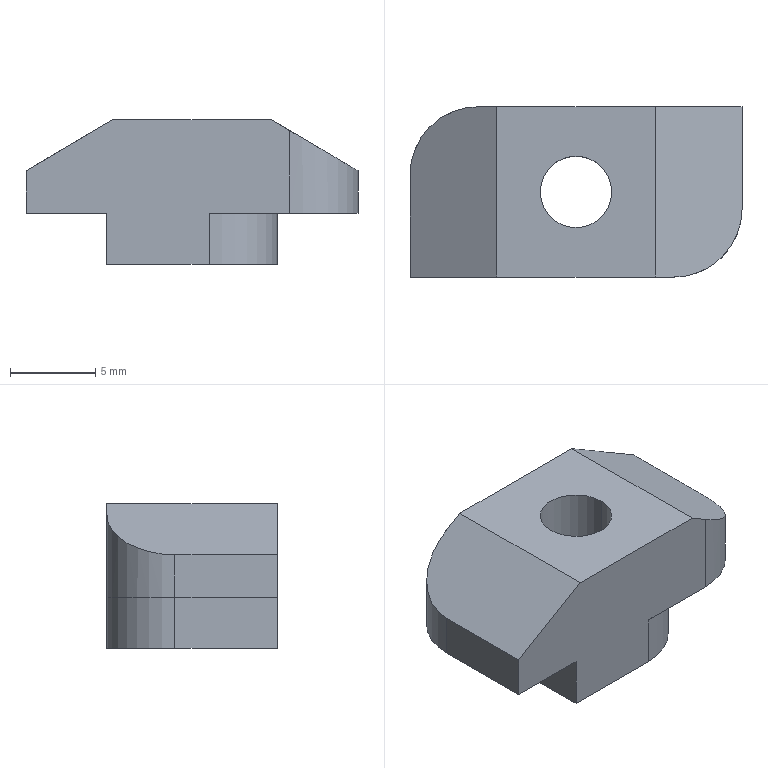Part | NX | features BREP 1 | 1 solid | 18 faces | box 19.5 x 10 x 8.5 mm | volume 1060 mm3 | plane 12 | cylinder 6 | commonest cylinder face diameters 8 x4 4.2 x2
STEP:
#1=CARTESIAN_POINT('',(-2.1,0.,-8.5));
#2=VERTEX_POINT('',#1);
#3=CARTESIAN_POINT('',(2.1,0.,-8.5));
#4=VERTEX_POINT('',#3);
#5=CARTESIAN_POINT('',(0.,0.,-8.5));
#6=DIRECTION('',(0.,0.,-1.));
#7=DIRECTION('',(-1.,0.,0.));
#8=AXIS2_PLACEMENT_3D('',#5,#6,#7);
#9=CIRCLE('',#8,2.1);
#10=EDGE_CURVE('',#2,#4,#9,.T.);
#11=ORIENTED_EDGE('',*,*,#10,.T.);
#12=CARTESIAN_POINT('',(2.1,0.,0.));
#13=VERTEX_POINT('',#12);
#14=CARTESIAN_POINT('',(2.1,0.,0.));
#15=DIRECTION('',(0.,0.,1.));
#16=VECTOR('',#15,1000.);
#17=LINE('',#14,#16);
#18=EDGE_CURVE('',#4,#13,#17,.T.);
#19=ORIENTED_EDGE('',*,*,#18,.T.);
#20=CARTESIAN_POINT('',(-2.1,0.,0.));
#21=VERTEX_POINT('',#20);
#22=CARTESIAN_POINT('',(0.,0.,0.));
#23=DIRECTION('',(0.,0.,-1.));
#24=DIRECTION('',(-1.,0.,0.));
#25=AXIS2_PLACEMENT_3D('',#22,#23,#24);
#26=CIRCLE('',#25,2.1);
#27=EDGE_CURVE('',#21,#13,#26,.T.);
#28=ORIENTED_EDGE('',*,*,#27,.F.);
#29=CARTESIAN_POINT('',(-2.1,0.,0.));
#30=DIRECTION('',(0.,0.,1.));
#31=VECTOR('',#30,1000.);
#32=LINE('',#29,#31);
#33=EDGE_CURVE('',#2,#21,#32,.T.);
#34=ORIENTED_EDGE('',*,*,#33,.F.);
#35=EDGE_LOOP('',(#11,#19,#28,#34));
#36=FACE_BOUND('',#35,.T.);
#37=CARTESIAN_POINT('',(0.,0.,0.));
#38=DIRECTION('',(0.,0.,1.));
#39=DIRECTION('',(-1.,0.,0.));
#40=AXIS2_PLACEMENT_3D('',#37,#38,#39);
#41=CYLINDRICAL_SURFACE('',#40,2.1);
#42=ADVANCED_FACE('',(#36),#41,.F.);
#43=CARTESIAN_POINT('',(1.,-5.,-5.5));
#44=VERTEX_POINT('',#43);
#45=CARTESIAN_POINT('',(5.75,-5.,-5.5));
#46=VERTEX_POINT('',#45);
#47=CARTESIAN_POINT('',(-9.75,-5.,-5.5));
#48=DIRECTION('',(1.,0.,0.));
#49=VECTOR('',#48,1000.);
#50=LINE('',#47,#49);
#51=EDGE_CURVE('',#44,#46,#50,.T.);
#52=ORIENTED_EDGE('',*,*,#51,.F.);
#53=CARTESIAN_POINT('',(5.,-1.,-5.5));
#54=VERTEX_POINT('',#53);
#55=CARTESIAN_POINT('',(1.,-1.,-5.5));
#56=DIRECTION('',(0.,0.,-1.));
#57=DIRECTION('',(1.,0.,0.));
#58=AXIS2_PLACEMENT_3D('',#55,#56,#57);
#59=CIRCLE('',#58,4.);
#60=EDGE_CURVE('',#54,#44,#59,.T.);
#61=ORIENTED_EDGE('',*,*,#60,.F.);
#62=CARTESIAN_POINT('',(5.,5.,-5.5));
#63=VERTEX_POINT('',#62);
#64=CARTESIAN_POINT('',(5.,-5.,-5.5));
#65=DIRECTION('',(0.,1.,0.));
#66=VECTOR('',#65,1000.);
#67=LINE('',#64,#66);
#68=EDGE_CURVE('',#54,#63,#67,.T.);
#69=ORIENTED_EDGE('',*,*,#68,.T.);
#70=CARTESIAN_POINT('',(9.75,5.,-5.5));
#71=VERTEX_POINT('',#70);
#72=CARTESIAN_POINT('',(-9.75,5.,-5.5));
#73=DIRECTION('',(-1.,0.,0.));
#74=VECTOR('',#73,1000.);
#75=LINE('',#72,#74);
#76=EDGE_CURVE('',#71,#63,#75,.T.);
#77=ORIENTED_EDGE('',*,*,#76,.F.);
#78=CARTESIAN_POINT('',(9.75,-1.,-5.5));
#79=VERTEX_POINT('',#78);
#80=CARTESIAN_POINT('',(9.75,5.,-5.5));
#81=DIRECTION('',(0.,1.,0.));
#82=VECTOR('',#81,1000.);
#83=LINE('',#80,#82);
#84=EDGE_CURVE('',#79,#71,#83,.T.);
#85=ORIENTED_EDGE('',*,*,#84,.F.);
#86=CARTESIAN_POINT('',(5.75,-1.,-5.5));
#87=DIRECTION('',(0.,0.,1.));
#88=DIRECTION('',(1.,0.,0.));
#89=AXIS2_PLACEMENT_3D('',#86,#87,#88);
#90=CIRCLE('',#89,4.);
#91=EDGE_CURVE('',#46,#79,#90,.T.);
#92=ORIENTED_EDGE('',*,*,#91,.F.);
#93=EDGE_LOOP('',(#52,#61,#69,#77,#85,#92));
#94=FACE_BOUND('',#93,.T.);
#95=CARTESIAN_POINT('',(0.,0.,-5.5));
#96=DIRECTION('',(0.,0.,-1.));
#97=DIRECTION('',(0.,-1.,0.));
#98=AXIS2_PLACEMENT_3D('',#95,#96,#97);
#99=PLANE('',#98);
#100=ADVANCED_FACE('',(#94),#99,.T.);
#101=ORIENTED_EDGE('',*,*,#84,.T.);
#102=CARTESIAN_POINT('',(9.75,5.,-3.));
#103=VERTEX_POINT('',#102);
#104=CARTESIAN_POINT('',(9.75,5.,-5.5));
#105=DIRECTION('',(0.,0.,1.));
#106=VECTOR('',#105,1000.);
#107=LINE('',#104,#106);
#108=EDGE_CURVE('',#71,#103,#107,.T.);
#109=ORIENTED_EDGE('',*,*,#108,.T.);
#110=CARTESIAN_POINT('',(9.75,-1.,-3.));
#111=VERTEX_POINT('',#110);
#112=CARTESIAN_POINT('',(9.75,5.,-3.));
#113=DIRECTION('',(0.,1.,0.));
#114=VECTOR('',#113,1000.);
#115=LINE('',#112,#114);
#116=EDGE_CURVE('',#111,#103,#115,.T.);
#117=ORIENTED_EDGE('',*,*,#116,.F.);
#118=CARTESIAN_POINT('',(9.75,-1.,-5.5));
#119=DIRECTION('',(0.,0.,1.));
#120=VECTOR('',#119,1000.);
#121=LINE('',#118,#120);
#122=EDGE_CURVE('',#79,#111,#121,.T.);
#123=ORIENTED_EDGE('',*,*,#122,.F.);
#124=EDGE_LOOP('',(#101,#109,#117,#123));
#125=FACE_BOUND('',#124,.T.);
#126=CARTESIAN_POINT('',(9.75,5.,-5.5));
#127=DIRECTION('',(-1.,0.,0.));
#128=DIRECTION('',(0.,1.,0.));
#129=AXIS2_PLACEMENT_3D('',#126,#127,#128);
#130=PLANE('',#129);
#131=ADVANCED_FACE('',(#125),#130,.F.);
#132=CARTESIAN_POINT('',(-4.65,5.,0.));
#133=VERTEX_POINT('',#132);
#134=CARTESIAN_POINT('',(-5.75,5.,-0.6471));
#135=VERTEX_POINT('',#134);
#136=CARTESIAN_POINT('',(-9.75,5.,-3.));
#137=DIRECTION('',(-0.8619,0.,-0.507));
#138=VECTOR('',#137,1000.);
#139=LINE('',#136,#138);
#140=EDGE_CURVE('',#133,#135,#139,.T.);
#141=ORIENTED_EDGE('',*,*,#140,.F.);
#142=CARTESIAN_POINT('',(4.65,5.,0.));
#143=VERTEX_POINT('',#142);
#144=CARTESIAN_POINT('',(-9.75,5.,0.));
#145=DIRECTION('',(-1.,0.,0.));
#146=VECTOR('',#145,1000.);
#147=LINE('',#144,#146);
#148=EDGE_CURVE('',#143,#133,#147,.T.);
#149=ORIENTED_EDGE('',*,*,#148,.F.);
#150=CARTESIAN_POINT('',(9.75,5.,-3.));
#151=DIRECTION('',(-0.8619,0.,0.507));
#152=VECTOR('',#151,1000.);
#153=LINE('',#150,#152);
#154=EDGE_CURVE('',#103,#143,#153,.T.);
#155=ORIENTED_EDGE('',*,*,#154,.F.);
#156=ORIENTED_EDGE('',*,*,#108,.F.);
#157=ORIENTED_EDGE('',*,*,#76,.T.);
#158=CARTESIAN_POINT('',(5.,5.,-8.5));
#159=VERTEX_POINT('',#158);
#160=CARTESIAN_POINT('',(5.,5.,-8.5));
#161=DIRECTION('',(0.,0.,1.));
#162=VECTOR('',#161,1000.);
#163=LINE('',#160,#162);
#164=EDGE_CURVE('',#159,#63,#163,.T.);
#165=ORIENTED_EDGE('',*,*,#164,.F.);
#166=CARTESIAN_POINT('',(-1.,5.,-8.5));
#167=VERTEX_POINT('',#166);
#168=CARTESIAN_POINT('',(-5.,5.,-8.5));
#169=DIRECTION('',(-1.,0.,0.));
#170=VECTOR('',#169,1000.);
#171=LINE('',#168,#170);
#172=EDGE_CURVE('',#159,#167,#171,.T.);
#173=ORIENTED_EDGE('',*,*,#172,.T.);
#174=CARTESIAN_POINT('',(-1.,5.,-5.5));
#175=VERTEX_POINT('',#174);
#176=CARTESIAN_POINT('',(-1.,5.,-5.5));
#177=DIRECTION('',(0.,0.,-1.));
#178=VECTOR('',#177,1000.);
#179=LINE('',#176,#178);
#180=EDGE_CURVE('',#175,#167,#179,.T.);
#181=ORIENTED_EDGE('',*,*,#180,.F.);
#182=CARTESIAN_POINT('',(-5.75,5.,-5.5));
#183=VERTEX_POINT('',#182);
#184=CARTESIAN_POINT('',(-9.75,5.,-5.5));
#185=DIRECTION('',(-1.,0.,0.));
#186=VECTOR('',#185,1000.);
#187=LINE('',#184,#186);
#188=EDGE_CURVE('',#175,#183,#187,.T.);
#189=ORIENTED_EDGE('',*,*,#188,.T.);
#190=CARTESIAN_POINT('',(-5.75,5.,-5.5));
#191=DIRECTION('',(0.,0.,-1.));
#192=VECTOR('',#191,1000.);
#193=LINE('',#190,#192);
#194=EDGE_CURVE('',#135,#183,#193,.T.);
#195=ORIENTED_EDGE('',*,*,#194,.F.);
#196=EDGE_LOOP('',(#141,#149,#155,#156,#157,#165,#173,#181,#189,#195));
#197=FACE_BOUND('',#196,.T.);
#198=CARTESIAN_POINT('',(-9.75,5.,-5.5));
#199=DIRECTION('',(0.,-1.,0.));
#200=DIRECTION('',(0.,0.,-1.));
#201=AXIS2_PLACEMENT_3D('',#198,#199,#200);
#202=PLANE('',#201);
#203=ADVANCED_FACE('',(#197),#202,.F.);
#204=CARTESIAN_POINT('',(-9.75,1.,-5.5));
#205=VERTEX_POINT('',#204);
#206=CARTESIAN_POINT('',(-9.75,-5.,-5.5));
#207=VERTEX_POINT('',#206);
#208=CARTESIAN_POINT('',(-9.75,5.,-5.5));
#209=DIRECTION('',(0.,-1.,0.));
#210=VECTOR('',#209,1000.);
#211=LINE('',#208,#210);
#212=EDGE_CURVE('',#205,#207,#211,.T.);
#213=ORIENTED_EDGE('',*,*,#212,.T.);
#214=CARTESIAN_POINT('',(-9.75,-5.,-3.));
#215=VERTEX_POINT('',#214);
#216=CARTESIAN_POINT('',(-9.75,-5.,-5.5));
#217=DIRECTION('',(0.,0.,1.));
#218=VECTOR('',#217,1000.);
#219=LINE('',#216,#218);
#220=EDGE_CURVE('',#207,#215,#219,.T.);
#221=ORIENTED_EDGE('',*,*,#220,.T.);
#222=CARTESIAN_POINT('',(-9.75,1.,-3.));
#223=VERTEX_POINT('',#222);
#224=CARTESIAN_POINT('',(-9.75,5.,-3.));
#225=DIRECTION('',(0.,-1.,0.));
#226=VECTOR('',#225,1000.);
#227=LINE('',#224,#226);
#228=EDGE_CURVE('',#223,#215,#227,.T.);
#229=ORIENTED_EDGE('',*,*,#228,.F.);
#230=CARTESIAN_POINT('',(-9.75,1.,-5.5));
#231=DIRECTION('',(0.,0.,1.));
#232=VECTOR('',#231,1000.);
#233=LINE('',#230,#232);
#234=EDGE_CURVE('',#205,#223,#233,.T.);
#235=ORIENTED_EDGE('',*,*,#234,.F.);
#236=EDGE_LOOP('',(#213,#221,#229,#235));
#237=FACE_BOUND('',#236,.T.);
#238=CARTESIAN_POINT('',(-9.75,5.,-5.5));
#239=DIRECTION('',(1.,0.,0.));
#240=DIRECTION('',(0.,1.,0.));
#241=AXIS2_PLACEMENT_3D('',#238,#239,#240);
#242=PLANE('',#241);
#243=ADVANCED_FACE('',(#237),#242,.F.);
#244=CARTESIAN_POINT('',(4.65,-5.,0.));
#245=VERTEX_POINT('',#244);
#246=CARTESIAN_POINT('',(5.75,-5.,-0.6471));
#247=VERTEX_POINT('',#246);
#248=CARTESIAN_POINT('',(9.75,-5.,-3.));
#249=DIRECTION('',(0.8619,0.,-0.507));
#250=VECTOR('',#249,1000.);
#251=LINE('',#248,#250);
#252=EDGE_CURVE('',#245,#247,#251,.T.);
#253=ORIENTED_EDGE('',*,*,#252,.F.);
#254=CARTESIAN_POINT('',(-4.65,-5.,0.));
#255=VERTEX_POINT('',#254);
#256=CARTESIAN_POINT('',(-9.75,-5.,0.));
#257=DIRECTION('',(1.,0.,0.));
#258=VECTOR('',#257,1000.);
#259=LINE('',#256,#258);
#260=EDGE_CURVE('',#255,#245,#259,.T.);
#261=ORIENTED_EDGE('',*,*,#260,.F.);
#262=CARTESIAN_POINT('',(-9.75,-5.,-3.));
#263=DIRECTION('',(0.8619,0.,0.507));
#264=VECTOR('',#263,1000.);
#265=LINE('',#262,#264);
#266=EDGE_CURVE('',#215,#255,#265,.T.);
#267=ORIENTED_EDGE('',*,*,#266,.F.);
#268=ORIENTED_EDGE('',*,*,#220,.F.);
#269=CARTESIAN_POINT('',(-5.,-5.,-5.5));
#270=VERTEX_POINT('',#269);
#271=CARTESIAN_POINT('',(-9.75,-5.,-5.5));
#272=DIRECTION('',(1.,0.,0.));
#273=VECTOR('',#272,1000.);
#274=LINE('',#271,#273);
#275=EDGE_CURVE('',#207,#270,#274,.T.);
#276=ORIENTED_EDGE('',*,*,#275,.T.);
#277=CARTESIAN_POINT('',(-5.,-5.,-8.5));
#278=VERTEX_POINT('',#277);
#279=CARTESIAN_POINT('',(-5.,-5.,-8.5));
#280=DIRECTION('',(0.,0.,1.));
#281=VECTOR('',#280,1000.);
#282=LINE('',#279,#281);
#283=EDGE_CURVE('',#278,#270,#282,.T.);
#284=ORIENTED_EDGE('',*,*,#283,.F.);
#285=CARTESIAN_POINT('',(1.,-5.,-8.5));
#286=VERTEX_POINT('',#285);
#287=CARTESIAN_POINT('',(-5.,-5.,-8.5));
#288=DIRECTION('',(1.,0.,0.));
#289=VECTOR('',#288,1000.);
#290=LINE('',#287,#289);
#291=EDGE_CURVE('',#278,#286,#290,.T.);
#292=ORIENTED_EDGE('',*,*,#291,.T.);
#293=CARTESIAN_POINT('',(1.,-5.,-5.5));
#294=DIRECTION('',(0.,0.,-1.));
#295=VECTOR('',#294,1000.);
#296=LINE('',#293,#295);
#297=EDGE_CURVE('',#44,#286,#296,.T.);
#298=ORIENTED_EDGE('',*,*,#297,.F.);
#299=ORIENTED_EDGE('',*,*,#51,.T.);
#300=CARTESIAN_POINT('',(5.75,-5.,-5.5));
#301=DIRECTION('',(0.,0.,-1.));
#302=VECTOR('',#301,1000.);
#303=LINE('',#300,#302);
#304=EDGE_CURVE('',#247,#46,#303,.T.);
#305=ORIENTED_EDGE('',*,*,#304,.F.);
#306=EDGE_LOOP('',(#253,#261,#267,#268,#276,#284,#292,#298,#299,#305));
#307=FACE_BOUND('',#306,.T.);
#308=CARTESIAN_POINT('',(-9.75,-5.,-5.5));
#309=DIRECTION('',(0.,1.,0.));
#310=DIRECTION('',(1.,0.,0.));
#311=AXIS2_PLACEMENT_3D('',#308,#309,#310);
#312=PLANE('',#311);
#313=ADVANCED_FACE('',(#307),#312,.F.);
#314=ORIENTED_EDGE('',*,*,#188,.F.);
#315=CARTESIAN_POINT('',(-5.,1.,-5.5));
#316=VERTEX_POINT('',#315);
#317=CARTESIAN_POINT('',(-1.,1.,-5.5));
#318=DIRECTION('',(0.,0.,-1.));
#319=DIRECTION('',(1.,0.,0.));
#320=AXIS2_PLACEMENT_3D('',#317,#318,#319);
#321=CIRCLE('',#320,4.);
#322=EDGE_CURVE('',#316,#175,#321,.T.);
#323=ORIENTED_EDGE('',*,*,#322,.F.);
#324=CARTESIAN_POINT('',(-5.,-5.,-5.5));
#325=DIRECTION('',(0.,-1.,0.));
#326=VECTOR('',#325,1000.);
#327=LINE('',#324,#326);
#328=EDGE_CURVE('',#316,#270,#327,.T.);
#329=ORIENTED_EDGE('',*,*,#328,.T.);
#330=ORIENTED_EDGE('',*,*,#275,.F.);
#331=ORIENTED_EDGE('',*,*,#212,.F.);
#332=CARTESIAN_POINT('',(-5.75,1.,-5.5));
#333=DIRECTION('',(0.,0.,1.));
#334=DIRECTION('',(1.,0.,0.));
#335=AXIS2_PLACEMENT_3D('',#332,#333,#334);
#336=CIRCLE('',#335,4.);
#337=EDGE_CURVE('',#183,#205,#336,.T.);
#338=ORIENTED_EDGE('',*,*,#337,.F.);
#339=EDGE_LOOP('',(#314,#323,#329,#330,#331,#338));
#340=FACE_BOUND('',#339,.T.);
#341=CARTESIAN_POINT('',(0.,0.,-5.5));
#342=DIRECTION('',(0.,0.,-1.));
#343=DIRECTION('',(0.,-1.,0.));
#344=AXIS2_PLACEMENT_3D('',#341,#342,#343);
#345=PLANE('',#344);
#346=ADVANCED_FACE('',(#340),#345,.T.);
#347=ORIENTED_EDGE('',*,*,#148,.T.);
#348=CARTESIAN_POINT('',(-4.65,0.,0.));
#349=DIRECTION('',(0.,1.,0.));
#350=VECTOR('',#349,1000.);
#351=LINE('',#348,#350);
#352=EDGE_CURVE('',#255,#133,#351,.T.);
#353=ORIENTED_EDGE('',*,*,#352,.F.);
#354=ORIENTED_EDGE('',*,*,#260,.T.);
#355=CARTESIAN_POINT('',(4.65,0.,0.));
#356=DIRECTION('',(0.,-1.,0.));
#357=VECTOR('',#356,1000.);
#358=LINE('',#355,#357);
#359=EDGE_CURVE('',#143,#245,#358,.T.);
#360=ORIENTED_EDGE('',*,*,#359,.F.);
#361=EDGE_LOOP('',(#347,#353,#354,#360));
#362=FACE_BOUND('',#361,.T.);
#363=ORIENTED_EDGE('',*,*,#27,.T.);
#364=CARTESIAN_POINT('',(0.,0.,0.));
#365=DIRECTION('',(0.,0.,-1.));
#366=DIRECTION('',(-1.,0.,0.));
#367=AXIS2_PLACEMENT_3D('',#364,#365,#366);
#368=CIRCLE('',#367,2.1);
#369=EDGE_CURVE('',#13,#21,#368,.T.);
#370=ORIENTED_EDGE('',*,*,#369,.T.);
#371=EDGE_LOOP('',(#363,#370));
#372=FACE_BOUND('',#371,.T.);
#373=CARTESIAN_POINT('',(0.,0.,0.));
#374=DIRECTION('',(0.,0.,-1.));
#375=DIRECTION('',(0.,-1.,0.));
#376=AXIS2_PLACEMENT_3D('',#373,#374,#375);
#377=PLANE('',#376);
#378=ADVANCED_FACE('',(#362,#372),#377,.F.);
#379=CARTESIAN_POINT('',(5.,-1.,-8.5));
#380=VERTEX_POINT('',#379);
#381=CARTESIAN_POINT('',(5.,-5.,-8.5));
#382=DIRECTION('',(0.,1.,0.));
#383=VECTOR('',#382,1000.);
#384=LINE('',#381,#383);
#385=EDGE_CURVE('',#380,#159,#384,.T.);
#386=ORIENTED_EDGE('',*,*,#385,.T.);
#387=ORIENTED_EDGE('',*,*,#164,.T.);
#388=ORIENTED_EDGE('',*,*,#68,.F.);
#389=CARTESIAN_POINT('',(5.,-1.,-8.5));
#390=DIRECTION('',(0.,0.,1.));
#391=VECTOR('',#390,1000.);
#392=LINE('',#389,#391);
#393=EDGE_CURVE('',#380,#54,#392,.T.);
#394=ORIENTED_EDGE('',*,*,#393,.F.);
#395=EDGE_LOOP('',(#386,#387,#388,#394));
#396=FACE_BOUND('',#395,.T.);
#397=CARTESIAN_POINT('',(5.,-5.,-8.5));
#398=DIRECTION('',(-1.,0.,0.));
#399=DIRECTION('',(0.,0.,1.));
#400=AXIS2_PLACEMENT_3D('',#397,#398,#399);
#401=PLANE('',#400);
#402=ADVANCED_FACE('',(#396),#401,.F.);
#403=CARTESIAN_POINT('',(-5.,1.,-8.5));
#404=VERTEX_POINT('',#403);
#405=CARTESIAN_POINT('',(-5.,-5.,-8.5));
#406=DIRECTION('',(0.,-1.,0.));
#407=VECTOR('',#406,1000.);
#408=LINE('',#405,#407);
#409=EDGE_CURVE('',#404,#278,#408,.T.);
#410=ORIENTED_EDGE('',*,*,#409,.T.);
#411=ORIENTED_EDGE('',*,*,#283,.T.);
#412=ORIENTED_EDGE('',*,*,#328,.F.);
#413=CARTESIAN_POINT('',(-5.,1.,-8.5));
#414=DIRECTION('',(0.,0.,1.));
#415=VECTOR('',#414,1000.);
#416=LINE('',#413,#415);
#417=EDGE_CURVE('',#404,#316,#416,.T.);
#418=ORIENTED_EDGE('',*,*,#417,.F.);
#419=EDGE_LOOP('',(#410,#411,#412,#418));
#420=FACE_BOUND('',#419,.T.);
#421=CARTESIAN_POINT('',(-5.,-5.,-8.5));
#422=DIRECTION('',(1.,0.,0.));
#423=DIRECTION('',(0.,1.,0.));
#424=AXIS2_PLACEMENT_3D('',#421,#422,#423);
#425=PLANE('',#424);
#426=ADVANCED_FACE('',(#420),#425,.F.);
#427=ORIENTED_EDGE('',*,*,#291,.F.);
#428=ORIENTED_EDGE('',*,*,#409,.F.);
#429=CARTESIAN_POINT('',(-1.,1.,-8.5));
#430=DIRECTION('',(0.,0.,1.));
#431=DIRECTION('',(-1.,0.,0.));
#432=AXIS2_PLACEMENT_3D('',#429,#430,#431);
#433=CIRCLE('',#432,4.);
#434=EDGE_CURVE('',#167,#404,#433,.T.);
#435=ORIENTED_EDGE('',*,*,#434,.F.);
#436=ORIENTED_EDGE('',*,*,#172,.F.);
#437=ORIENTED_EDGE('',*,*,#385,.F.);
#438=CARTESIAN_POINT('',(1.,-1.,-8.5));
#439=DIRECTION('',(0.,0.,1.));
#440=DIRECTION('',(-1.,0.,0.));
#441=AXIS2_PLACEMENT_3D('',#438,#439,#440);
#442=CIRCLE('',#441,4.);
#443=EDGE_CURVE('',#286,#380,#442,.T.);
#444=ORIENTED_EDGE('',*,*,#443,.F.);
#445=EDGE_LOOP('',(#427,#428,#435,#436,#437,#444));
#446=FACE_BOUND('',#445,.T.);
#447=ORIENTED_EDGE('',*,*,#10,.F.);
#448=CARTESIAN_POINT('',(0.,0.,-8.5));
#449=DIRECTION('',(0.,0.,-1.));
#450=DIRECTION('',(-1.,0.,0.));
#451=AXIS2_PLACEMENT_3D('',#448,#449,#450);
#452=CIRCLE('',#451,2.1);
#453=EDGE_CURVE('',#4,#2,#452,.T.);
#454=ORIENTED_EDGE('',*,*,#453,.F.);
#455=EDGE_LOOP('',(#447,#454));
#456=FACE_BOUND('',#455,.T.);
#457=CARTESIAN_POINT('',(0.,0.,-8.5));
#458=DIRECTION('',(0.,0.,1.));
#459=DIRECTION('',(1.,0.,0.));
#460=AXIS2_PLACEMENT_3D('',#457,#458,#459);
#461=PLANE('',#460);
#462=ADVANCED_FACE('',(#446,#456),#461,.F.);
#463=ORIENTED_EDGE('',*,*,#18,.F.);
#464=ORIENTED_EDGE('',*,*,#453,.T.);
#465=ORIENTED_EDGE('',*,*,#33,.T.);
#466=ORIENTED_EDGE('',*,*,#369,.F.);
#467=EDGE_LOOP('',(#463,#464,#465,#466));
#468=FACE_BOUND('',#467,.T.);
#469=CARTESIAN_POINT('',(0.,0.,0.));
#470=DIRECTION('',(0.,0.,1.));
#471=DIRECTION('',(-1.,0.,0.));
#472=AXIS2_PLACEMENT_3D('',#469,#470,#471);
#473=CYLINDRICAL_SURFACE('',#472,2.1);
#474=ADVANCED_FACE('',(#468),#473,.F.);
#475=ORIENTED_EDGE('',*,*,#116,.T.);
#476=ORIENTED_EDGE('',*,*,#154,.T.);
#477=ORIENTED_EDGE('',*,*,#359,.T.);
#478=ORIENTED_EDGE('',*,*,#252,.T.);
#479=CARTESIAN_POINT('',(9.75,-1.,-3.));
#480=CARTESIAN_POINT('',(9.75,-3.343,-3.));
#481=CARTESIAN_POINT('',(8.093,-5.,-2.025));
#482=CARTESIAN_POINT('',(5.75,-5.,-0.6471));
#483=(BOUNDED_CURVE()B_SPLINE_CURVE(3,(#479,#480,#481,#482),.UNSPECIFIED.,.F.,.F.)B_SPLINE_CURVE_WITH_KNOTS((4,4),(3.142,4.712),.UNSPECIFIED.)CURVE()GEOMETRIC_REPRESENTATION_ITEM()RATIONAL_B_SPLINE_CURVE((1.,0.8047,0.8047,1.))REPRESENTATION_ITEM(''));
#484=EDGE_CURVE('',#111,#247,#483,.T.);
#485=ORIENTED_EDGE('',*,*,#484,.F.);
#486=EDGE_LOOP('',(#475,#476,#477,#478,#485));
#487=FACE_BOUND('',#486,.T.);
#488=CARTESIAN_POINT('',(9.75,5.,-3.));
#489=DIRECTION('',(-0.507,0.,-0.8619));
#490=DIRECTION('',(-0.8619,0.,0.507));
#491=AXIS2_PLACEMENT_3D('',#488,#489,#490);
#492=PLANE('',#491);
#493=ADVANCED_FACE('',(#487),#492,.F.);
#494=ORIENTED_EDGE('',*,*,#228,.T.);
#495=ORIENTED_EDGE('',*,*,#266,.T.);
#496=ORIENTED_EDGE('',*,*,#352,.T.);
#497=ORIENTED_EDGE('',*,*,#140,.T.);
#498=CARTESIAN_POINT('',(-9.75,1.,-3.));
#499=CARTESIAN_POINT('',(-9.75,3.343,-3.));
#500=CARTESIAN_POINT('',(-8.093,5.,-2.025));
#501=CARTESIAN_POINT('',(-5.75,5.,-0.6471));
#502=(BOUNDED_CURVE()B_SPLINE_CURVE(3,(#498,#499,#500,#501),.UNSPECIFIED.,.F.,.F.)B_SPLINE_CURVE_WITH_KNOTS((4,4),(3.142,4.712),.UNSPECIFIED.)CURVE()GEOMETRIC_REPRESENTATION_ITEM()RATIONAL_B_SPLINE_CURVE((1.,0.8047,0.8047,1.))REPRESENTATION_ITEM(''));
#503=EDGE_CURVE('',#223,#135,#502,.T.);
#504=ORIENTED_EDGE('',*,*,#503,.F.);
#505=EDGE_LOOP('',(#494,#495,#496,#497,#504));
#506=FACE_BOUND('',#505,.T.);
#507=CARTESIAN_POINT('',(-9.75,5.,-3.));
#508=DIRECTION('',(0.507,0.,-0.8619));
#509=DIRECTION('',(0.,-1.,0.));
#510=AXIS2_PLACEMENT_3D('',#507,#508,#509);
#511=PLANE('',#510);
#512=ADVANCED_FACE('',(#506),#511,.F.);
#513=ORIENTED_EDGE('',*,*,#443,.T.);
#514=ORIENTED_EDGE('',*,*,#393,.T.);
#515=ORIENTED_EDGE('',*,*,#60,.T.);
#516=ORIENTED_EDGE('',*,*,#297,.T.);
#517=EDGE_LOOP('',(#513,#514,#515,#516));
#518=FACE_BOUND('',#517,.T.);
#519=CARTESIAN_POINT('',(1.,-1.,-8.5));
#520=DIRECTION('',(0.,0.,1.));
#521=DIRECTION('',(-1.,0.,0.));
#522=AXIS2_PLACEMENT_3D('',#519,#520,#521);
#523=CYLINDRICAL_SURFACE('',#522,4.);
#524=ADVANCED_FACE('',(#518),#523,.T.);
#525=ORIENTED_EDGE('',*,*,#434,.T.);
#526=ORIENTED_EDGE('',*,*,#417,.T.);
#527=ORIENTED_EDGE('',*,*,#322,.T.);
#528=ORIENTED_EDGE('',*,*,#180,.T.);
#529=EDGE_LOOP('',(#525,#526,#527,#528));
#530=FACE_BOUND('',#529,.T.);
#531=CARTESIAN_POINT('',(-1.,1.,-8.5));
#532=DIRECTION('',(0.,0.,1.));
#533=DIRECTION('',(-1.,0.,0.));
#534=AXIS2_PLACEMENT_3D('',#531,#532,#533);
#535=CYLINDRICAL_SURFACE('',#534,4.);
#536=ADVANCED_FACE('',(#530),#535,.T.);
#537=ORIENTED_EDGE('',*,*,#91,.T.);
#538=ORIENTED_EDGE('',*,*,#122,.T.);
#539=ORIENTED_EDGE('',*,*,#484,.T.);
#540=ORIENTED_EDGE('',*,*,#304,.T.);
#541=EDGE_LOOP('',(#537,#538,#539,#540));
#542=FACE_BOUND('',#541,.T.);
#543=CARTESIAN_POINT('',(5.75,-1.,-5.5));
#544=DIRECTION('',(0.,0.,1.));
#545=DIRECTION('',(-1.,0.,0.));
#546=AXIS2_PLACEMENT_3D('',#543,#544,#545);
#547=CYLINDRICAL_SURFACE('',#546,4.);
#548=ADVANCED_FACE('',(#542),#547,.T.);
#549=ORIENTED_EDGE('',*,*,#337,.T.);
#550=ORIENTED_EDGE('',*,*,#234,.T.);
#551=ORIENTED_EDGE('',*,*,#503,.T.);
#552=ORIENTED_EDGE('',*,*,#194,.T.);
#553=EDGE_LOOP('',(#549,#550,#551,#552));
#554=FACE_BOUND('',#553,.T.);
#555=CARTESIAN_POINT('',(-5.75,1.,-5.5));
#556=DIRECTION('',(0.,0.,1.));
#557=DIRECTION('',(-1.,0.,0.));
#558=AXIS2_PLACEMENT_3D('',#555,#556,#557);
#559=CYLINDRICAL_SURFACE('',#558,4.);
#560=ADVANCED_FACE('',(#554),#559,.T.);
#561=CLOSED_SHELL('',(#42,#100,#131,#203,#243,#313,#346,#378,#402,#426,#462,#474,#493,#512,#524,#536,#548,#560));
#562=MANIFOLD_SOLID_BREP('',#561);
#563=(LENGTH_UNIT()NAMED_UNIT(*)SI_UNIT(.MILLI.,.METRE.));
#564=UNCERTAINTY_MEASURE_WITH_UNIT(LENGTH_MEASURE(0.00001),#563,'','');
#565=(NAMED_UNIT(*)PLANE_ANGLE_UNIT()SI_UNIT($,.RADIAN.));
#566=(NAMED_UNIT(*)SI_UNIT($,.STERADIAN.)SOLID_ANGLE_UNIT());
#567=(GEOMETRIC_REPRESENTATION_CONTEXT(3)GLOBAL_UNCERTAINTY_ASSIGNED_CONTEXT((#564))GLOBAL_UNIT_ASSIGNED_CONTEXT((#563,#565,#566))REPRESENTATION_CONTEXT('',''));
#568=ADVANCED_BREP_SHAPE_REPRESENTATION('',(#562),#567);